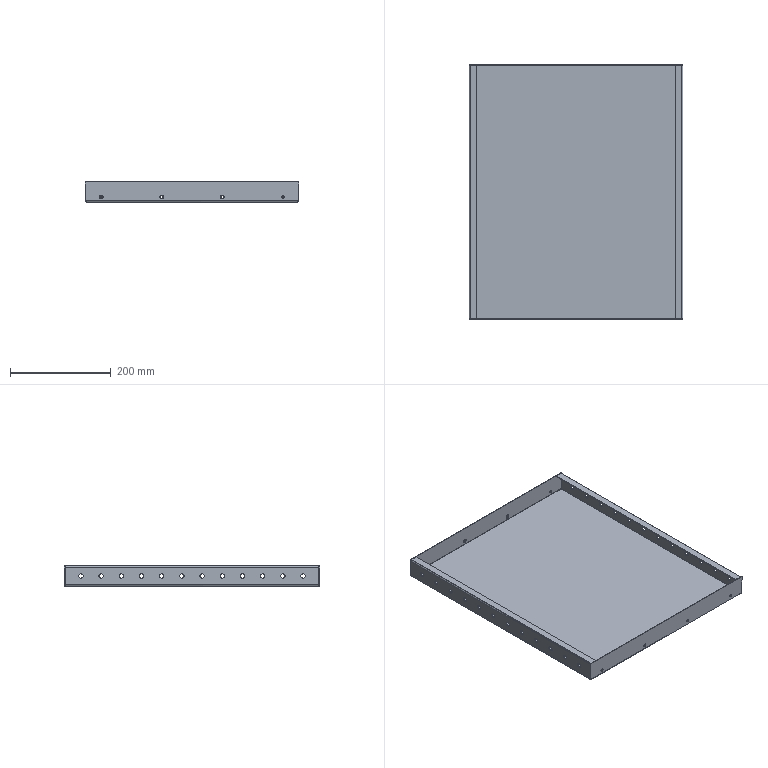Part | SolidWorks | features ICE 3, EdgeFlange 2, Chamfer 1, CornerFeat 1, FlatPattern 1, LPattern 1, SMBaseFlange 1, SheetMetal 1 | 1 solid | 138 faces | box 423 x 507 x 40 mm | volume 588577 mm3 | cylinder 76 | plane 42 | cone 12 | spline 8 | commonest cylinder face diameters 8.8 x48 5 x22 1 x6